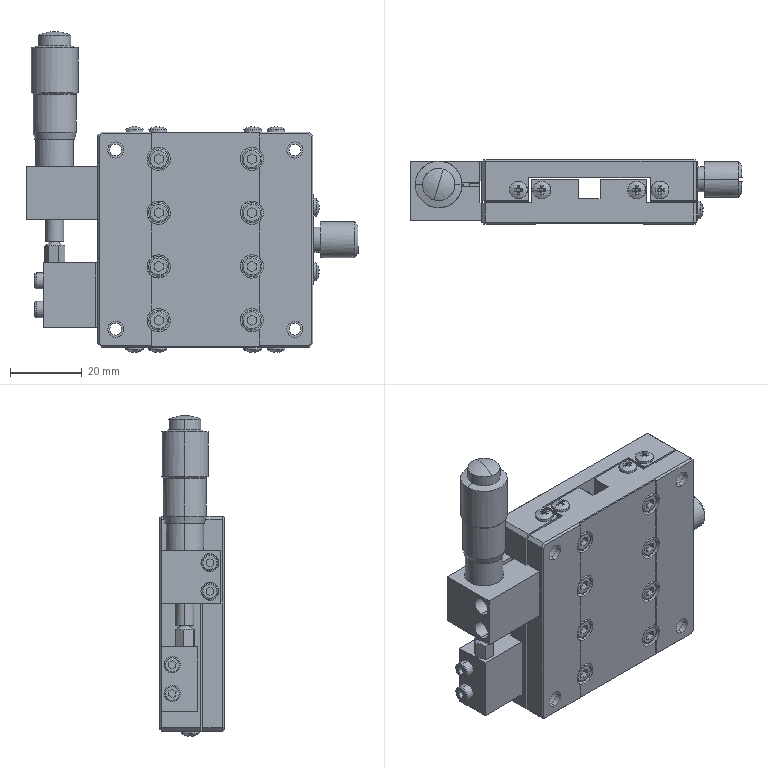Part | SolidWorks | features BaseBody 1 | 1 solid | 787 faces | box 92.6 x 18 x 89.45 mm | volume 68470 mm3 | plane 465 | cylinder 164 | cone 95 | spline 63 | commonest cylinder face diameters 5.5 x34 3.3 x18 6 x18 4.5 x16 6.5 x16 3 x10